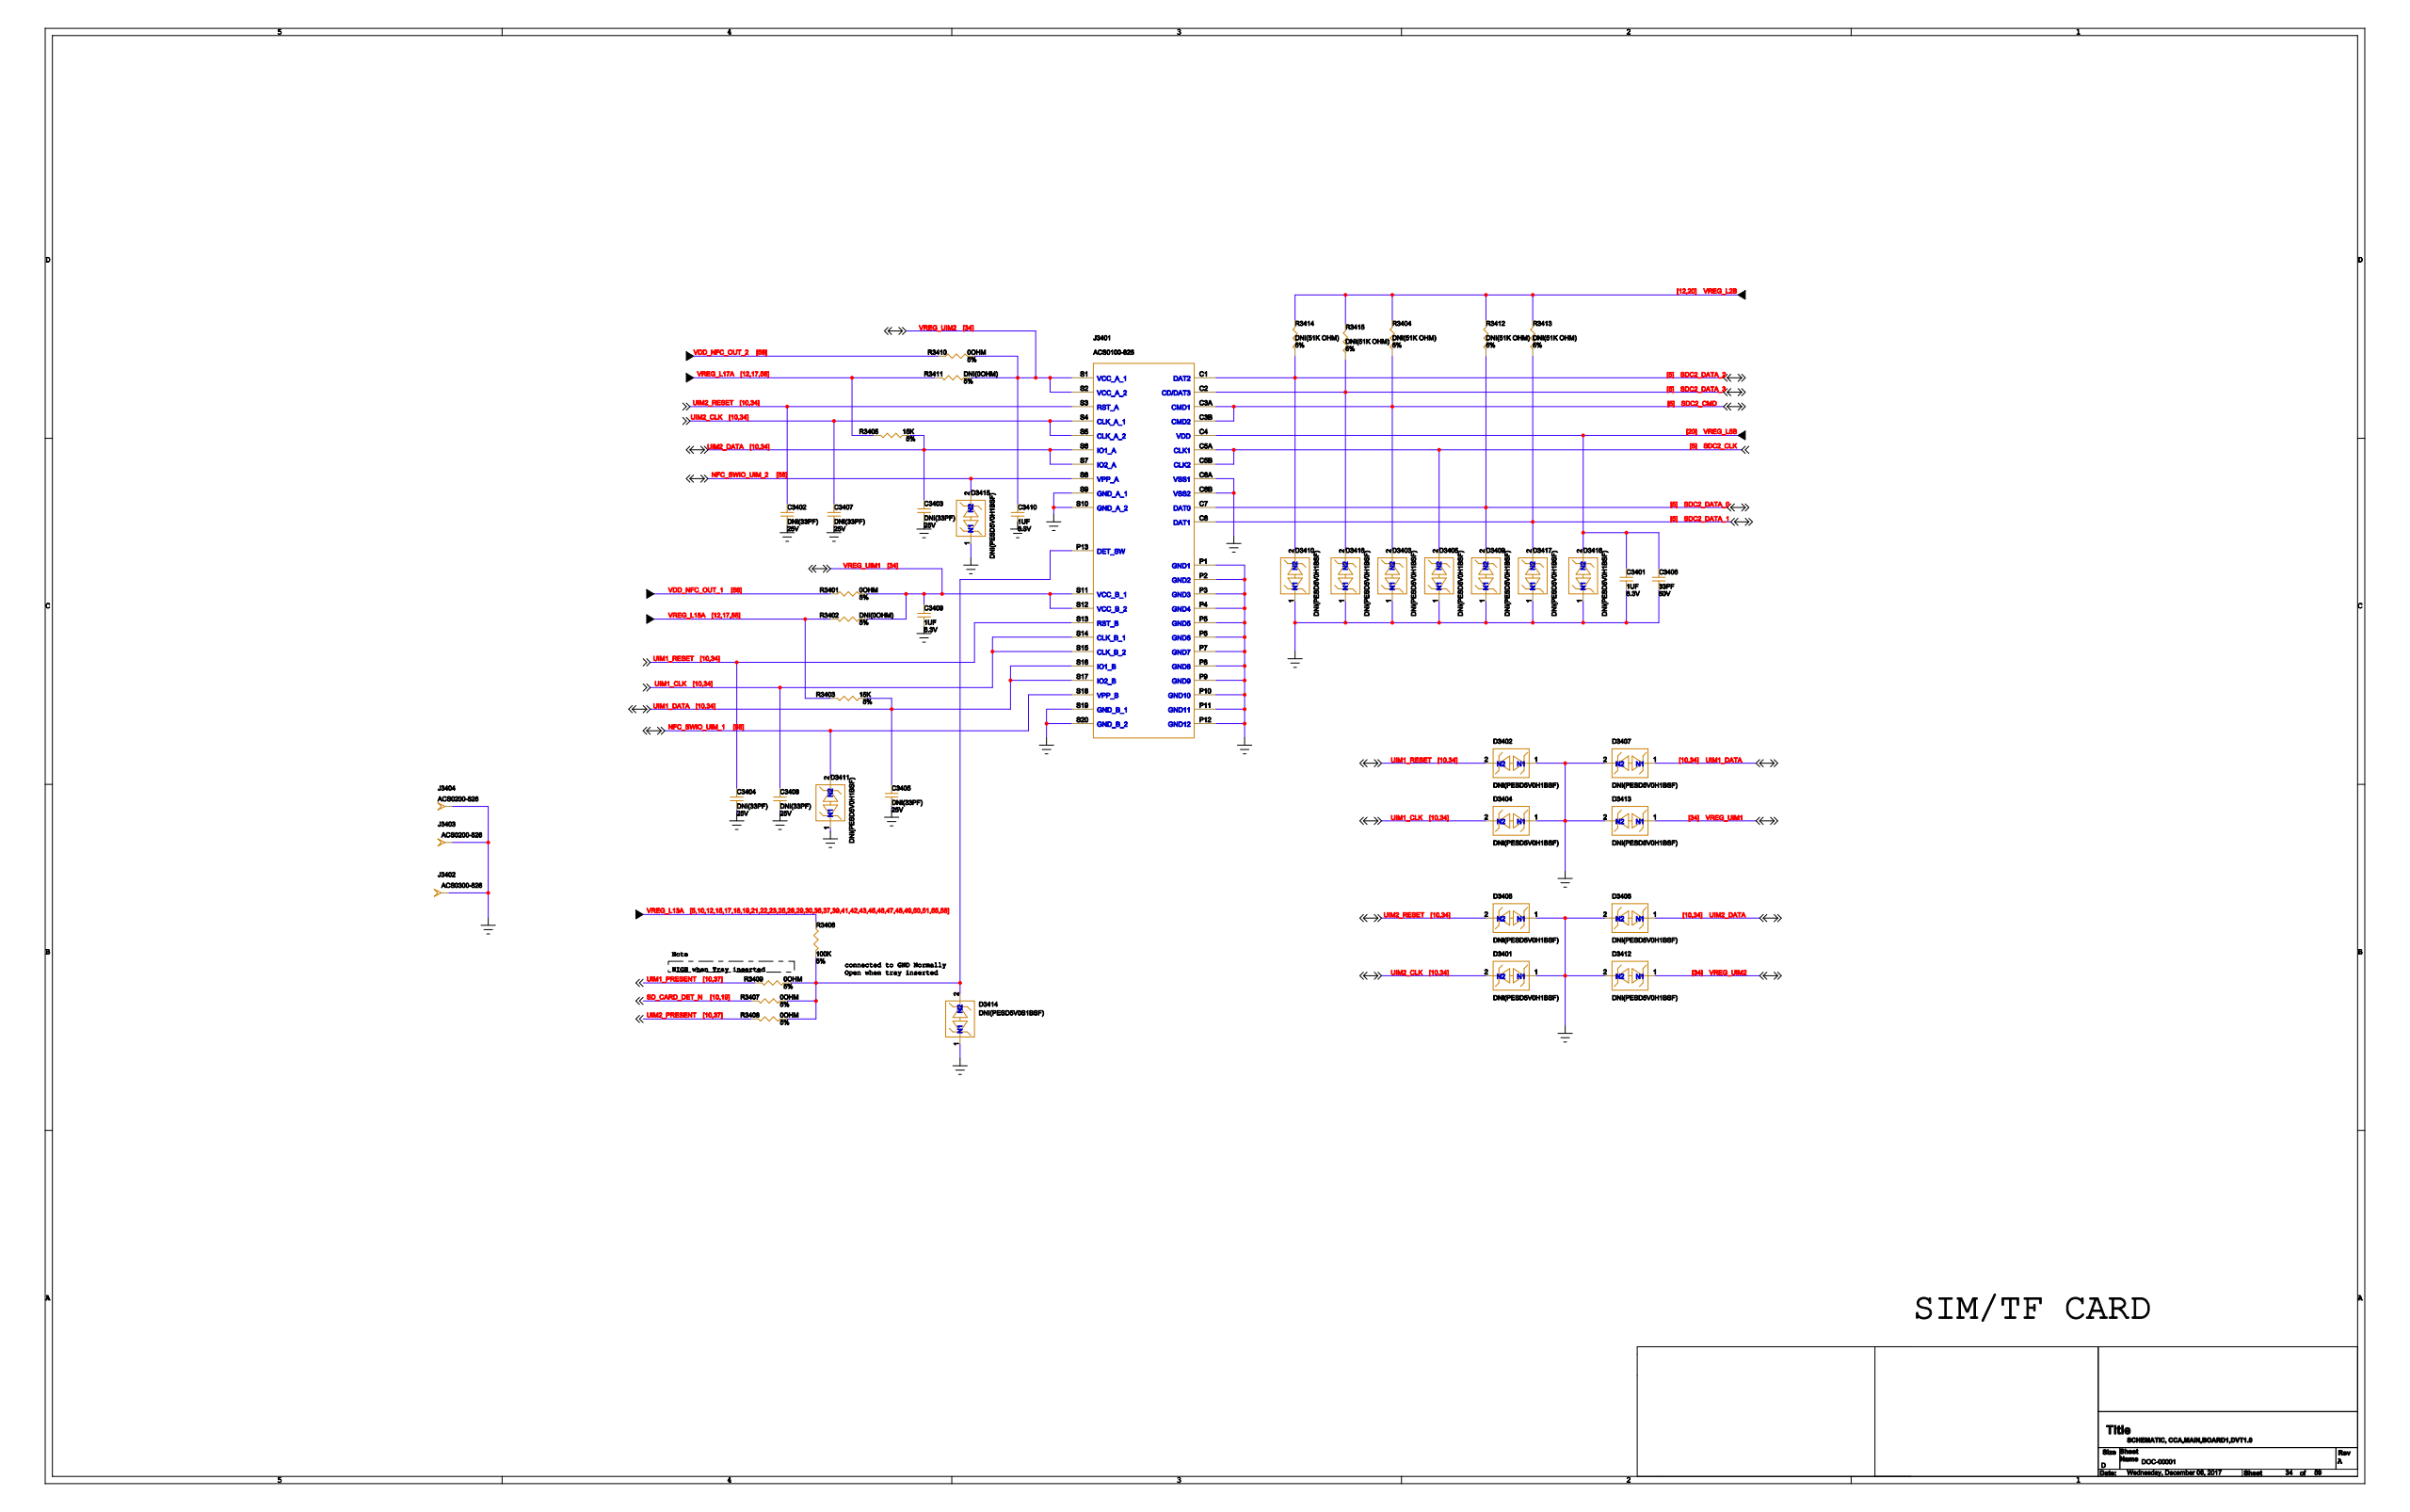Circuit board | KiCad | 1657 parts | 1365 nets | one sheet of the schematic
Parts on this sheet (reference | value | footprint):
C3401
C3402
C3403
C3404
C3405
C3406
C3407
C3408
C3409
C3410
D3401
D3402
D3403
D3404
D3405
D3406
D3407
D3408
D3409
D3410
D3411
D3412
D3413
D3414
D3415
D3416
D3417
D3418
J3401
J3402
J3403
J3404
R3401
R3402
R3403
R3404
R3405
R3406
R3407
R3408
R3409
R3410
R3411
R3412
R3413
R3414
R3415
Nets of these parts (net: part-pin ...):
GND: C3401-2 C3402-2 C3403-2 C3404-2 C3405-2 C3406-2 C3407-2 C3408-2 C3409-2 C3410-2 D3401-1 D3402-1 D3403-1 D3404-1 D3405-1 D3406-2 D3407-2 D3408-1 D3409-1 D3410-1 D3411-1 D3412-2 D3413-2 D3414-1 D3415-1 D3416-1 D3417-1 D3418-1 J3402-1 J3403-1 J3404-1 J3401-C6A J3401-C6B J3401-P1 J3401-P2 J3401-P3 J3401-P4 J3401-P5 J3401-P6 J3401-P7 J3401-P8 J3401-P9 J3401-P10 J3401-P11 J3401-P12 J3401-S9 J3401-S10 J3401-S19 J3401-S20
VREG_L13A: R3406-2
UIM1_CLK: C3408-1 D3404-2 J3401-S14 J3401-S15
SD_CARD_DET_N: R3407-1
N20342648: D3414-2 R3406-1 R3407-2 R3408-2 R3409-2 J3401-P13
VREG_L2B: R3404-1 R3412-1 R3413-1 R3414-1 R3415-1
UIM2_CLK: C3407-1 D3401-2 J3401-S4 J3401-S5
SDC2_DATA_3: D3416-2 R3415-2 J3401-C2
UIM2_RESET: C3402-1 D3408-2 J3401-S3
VREG_UIM2: C3410-1 D3412-1 R3410-1 R3411-2 J3401-S1 J3401-S2
SDC2_DATA_2: D3410-2 R3414-2 J3401-C1
SDC2_CMD: D3403-2 R3404-2 J3401-C3A J3401-C3B
VREG_L17A: R3405-1 R3411-1
VREG_L5B: C3401-1 C3406-1 D3418-2 J3401-C4
UIM1_RESET: C3404-1 D3402-2 J3401-S13
VREG_UIM1: C3409-1 D3413-1 R3401-1 R3402-2 J3401-S11 J3401-S12
UIM1_PRESENT: R3409-1
UIM2_DATA: C3403-1 D3406-1 R3405-2 J3401-S6 J3401-S7
UIM1_DATA: C3405-1 D3407-1 R3403-2 J3401-S16 J3401-S17
SDC2_DATA_1: D3417-2 R3413-2 J3401-C8
VDD_NFC_OUT_2: R3410-2
SDC2_DATA_0: D3409-2 R3412-2 J3401-C7
VREG_L15A: R3402-1 R3403-1
NFC_SWIO_UIM_2: D3415-2 J3401-S8
UIM2_PRESENT: R3408-1
VDD_NFC_OUT_1: R3401-2
SDC2_CLK: D3405-2 J3401-C5A J3401-C5B
NFC_SWIO_UIM_1: D3411-2 J3401-S18